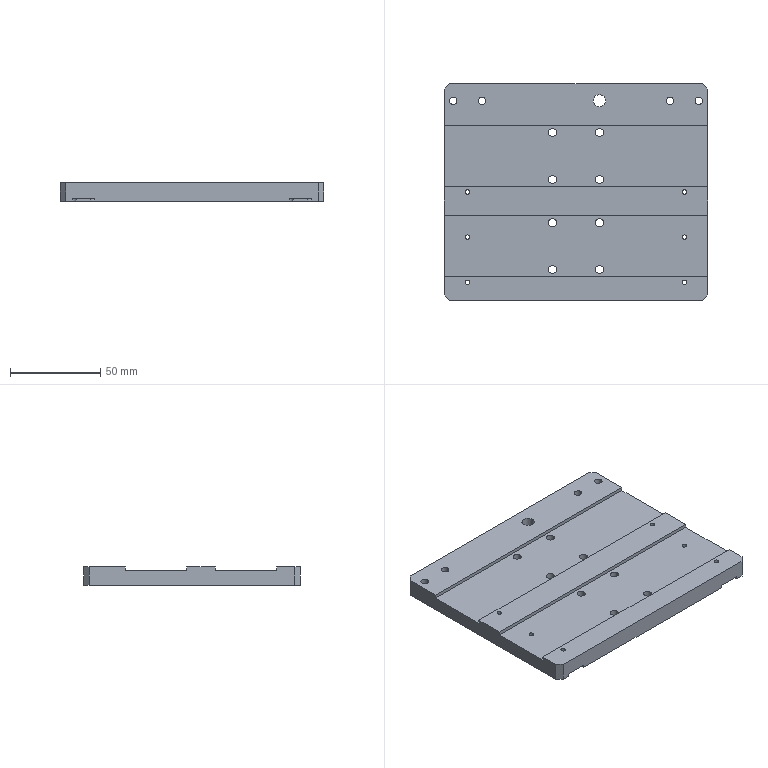Part | STEP file | A04 | 1 solid | 94 faces | box 146 x 120 x 10 mm | volume 149212 mm3 | cylinder 60 | plane 34 | commonest cylinder face diameters 4.5 x16 8 x16 2.5 x12 4.2 x8 4 x6 6.8 x2